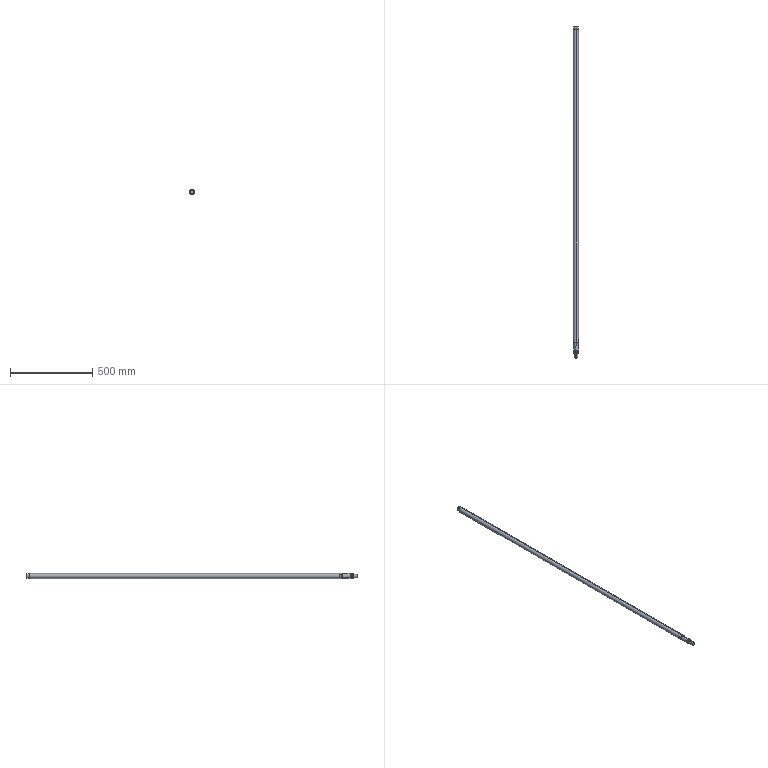Part | STEP file | 1 solid | 155 faces | box 31 x 2020 x 31 mm | volume 1487693 mm3 | cylinder 127 | plane 18 | cone 7 | spline 3 | commonest cylinder face diameters 25 x119 6 x2 20 x2 23.9 x2 31 x2